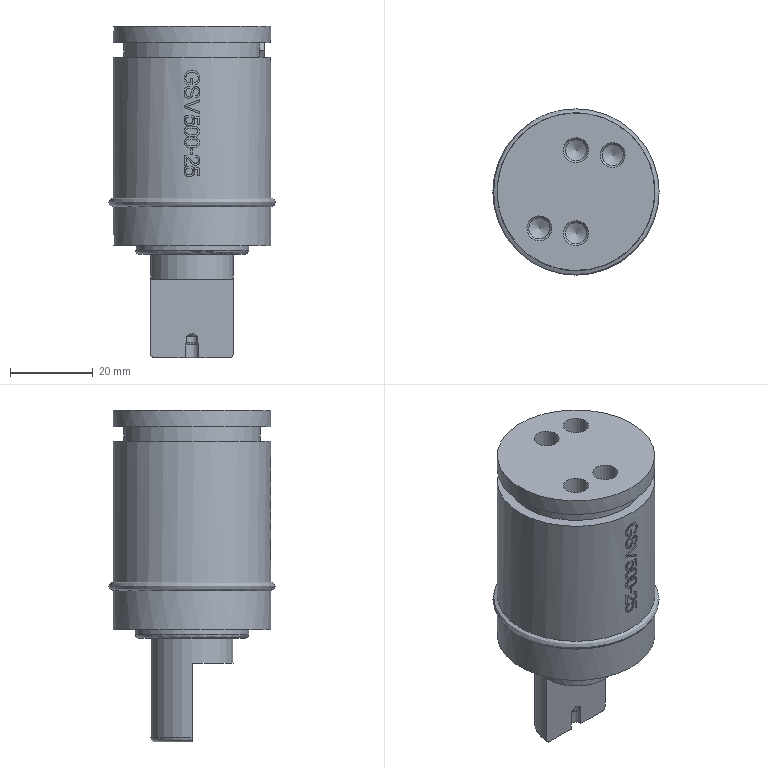Part | NX | features solid 2 | 1 solid | 187 faces | box 40.1 x 40.1 x 80 mm | volume 64413 mm3 | plane 96 | cylinder 78 | cone 10 | torus 2 | spline 1 | commonest cylinder face diameters 37.8 x9 6 x5 38 x5 5.1 x4 1.51 x2 1.588 x2